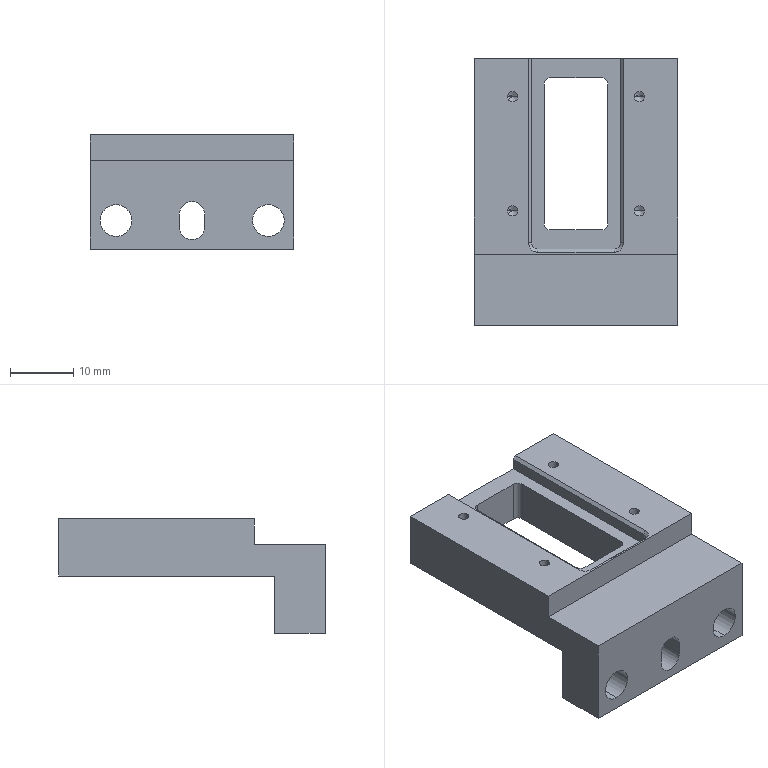NC program | NX | posted with a generic post | part box 32 x 42 x 18 mm
Whole program:
N10 G17 G21 G94 G90
(DRILLING_COPY_1 , TOOL : D6A45)
N12 T07 M6
N14 G54
N16 G17 G0 G90 X-11.974 Y4.5 B0. C0. S5000 M3
N18 G43 Z30. H7
N20 G94 G81 G98 Z-1. F250. R3.
N22 X12.026
N24 G80
N26 G0 X12.026 Y4.5 Z30.
N28 M5
(DRILLING_COPY_COPY , TOOL : 5.0ZT)
N30 T13 M6
N32 G54
N34 G17 G0 G90 X-11.974 Y4.5 B0. C0. S2000 M3
N36 G43 Z30. H13
N38 G94 G83 G98 Z-11.002 F200. Q2. R3.
N40 X12.026
N42 G80
N44 G0 X12.026 Y4.5 Z30.
N46 M5
(刀补3 , TOOL : D3)
N48 T03 M6
N50 G54
N52 G17 G0 G90 X0.113 Y3.402 B0. C0. S9500 M3
N54 G43 Z30. H3
N56 Z-1.
N58 G94 G1 Z-2. F1000.
N60 G41 X0.3 Y3.24 D3
N62 G3 X0.45 Y3.5 R0.3
N64 G1 Y5.5 F1200.
N66 G3 X0. Y5.95 R0.45
N68 X-0.45 Y5.5 R0.45
N70 G1 Y3.5
N72 G3 X0. Y3.05 R0.45
N74 X0.45 Y3.5 R0.45
N76 G1 Y5.329 Z-2.714
N78 X0.448 Y5.451 Z-2.762
N80 X0.437 Y5.569 Z-2.808
N82 X0.423 Y5.625 Z-2.831
N84 X0.402 Y5.685 Z-2.857
N86 X0.351 Y5.767 Z-2.895
N88 X0.322 Y5.804 Z-2.914
N90 X0.299 Y5.826 Z-2.927
N92 X0.249 Y5.866 Z-2.952
N94 X0.156 Y5.922 Z-2.993
N96 X0.107 Y5.937 Z-3.014
N98 X0.08 Y5.943 Z-3.025
N100 X0.025 Y5.949 Z-3.048
N102 X-0.068 Y5.945 Z-3.084
N104 X-0.143 Y5.917 Z-3.115
N106 X-0.206 Y5.889 Z-3.143
N108 X-0.289 Y5.834 Z-3.182
N110 X-0.325 Y5.801 Z-3.201
N112 X-0.344 Y5.778 Z-3.214
N114 X-0.379 Y5.728 Z-3.238
N116 X-0.411 Y5.667 Z-3.266
N118 X-0.434 Y5.591 Z-3.297
N120 X-0.444 Y5.5 Z-3.333
N122 X-0.45 Y5.378 Z-3.381
N124 Y3.793 Z-4.
N126 Y3.5
N128 G3 X0. Y3.05 R0.45
N130 X0.45 Y3.5 R0.45
N132 G1 Y5.329 Z-4.714
N134 X0.448 Y5.451 Z-4.762
N136 X0.437 Y5.569 Z-4.808
N138 X0.423 Y5.626 Z-4.832
N140 X0.402 Y5.685 Z-4.857
N142 X0.351 Y5.767 Z-4.895
N144 X0.322 Y5.804 Z-4.914
N146 X0.299 Y5.826 Z-4.927
N148 X0.249 Y5.866 Z-4.952
N150 X0.156 Y5.922 Z-4.993
N152 X0.107 Y5.937 Z-5.014
N154 X0.08 Y5.943 Z-5.025
N156 X0.025 Y5.949 Z-5.048
N158 X-0.068 Y5.945 Z-5.084
N160 X-0.143 Y5.917 Z-5.115
N162 X-0.206 Y5.889 Z-5.143
N164 X-0.289 Y5.834 Z-5.182
N166 X-0.325 Y5.801 Z-5.201
N168 X-0.344 Y5.778 Z-5.214
N170 X-0.379 Y5.728 Z-5.238
N172 X-0.411 Y5.667 Z-5.265
N174 X-0.434 Y5.591 Z-5.297
N176 X-0.444 Y5.5 Z-5.333
N178 X-0.45 Y5.378 Z-5.381
N180 Y3.793 Z-6.
N182 Y3.5
N184 G3 X0. Y3.05 R0.45
N186 X0.45 Y3.5 R0.45
N188 G1 Y5.329 Z-6.714
N190 X0.448 Y5.451 Z-6.762
N192 X0.437 Y5.569 Z-6.808
N194 X0.423 Y5.626 Z-6.832
N196 X0.402 Y5.685 Z-6.857
N198 X0.351 Y5.767 Z-6.895
N200 X0.322 Y5.804 Z-6.914
N202 X0.299 Y5.826 Z-6.927
N204 X0.249 Y5.866 Z-6.952
N206 X0.156 Y5.922 Z-6.993
N208 X0.107 Y5.937 Z-7.014
N210 X0.08 Y5.943 Z-7.025
N212 X0.025 Y5.949 Z-7.048
N214 X-0.068 Y5.945 Z-7.084
N216 X-0.143 Y5.917 Z-7.115
N218 X-0.206 Y5.889 Z-7.143
N220 X-0.289 Y5.834 Z-7.182
N222 X-0.325 Y5.801 Z-7.201
N224 X-0.344 Y5.778 Z-7.214
N226 X-0.379 Y5.728 Z-7.238
N228 X-0.411 Y5.667 Z-7.265
N230 X-0.434 Y5.591 Z-7.297
N232 X-0.444 Y5.5 Z-7.333
N234 X-0.45 Y5.378 Z-7.381
N236 Y3.793 Z-8.
N238 Y3.5
N240 G3 X0. Y3.05 R0.45
N242 X0.45 Y3.5 R0.45
N244 G1 Y5.5
N246 G3 X0. Y5.95 R0.45
N248 X-0.45 Y5.5 R0.45
N250 G1 Y3.793
N252 G3 X-0.3 Y3.533 R0.3
N254 G1 X-0.137 Y3.439
N256 G40
N258 X-0.043 Y3.405
N260 Z-7.
N262 G0 Z30.
N264 M5
N266 M2